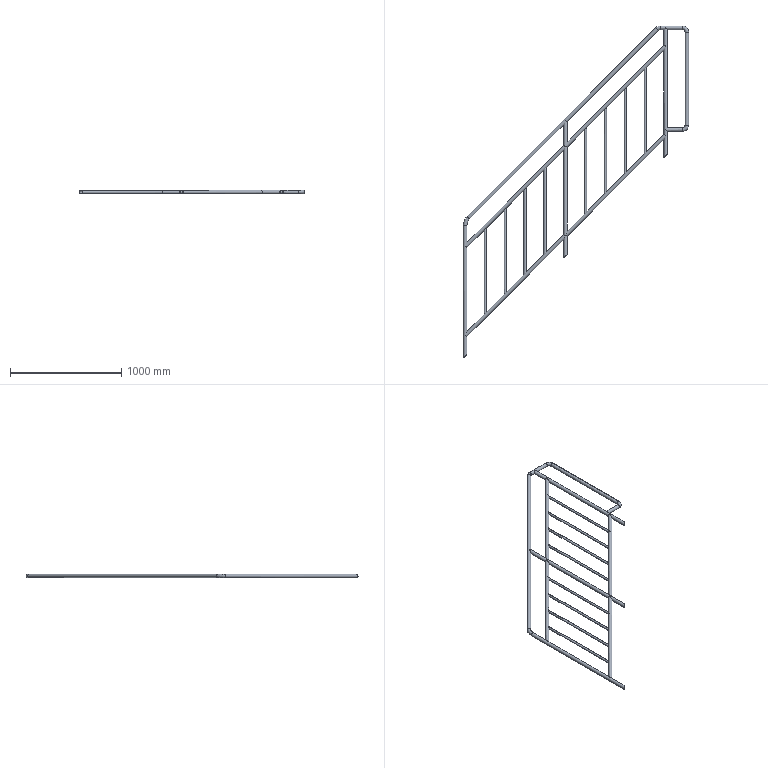Part | STEP file | PN_0012 stair guardrail B_Default<As Machined> | 23 solids | 92 faces | box 2022 x 2980 x 32 mm | volume 3009194 mm3 | cylinder 61 | plane 23 | torus 8 | commonest cylinder face diameters 32 x34 28 x11 16 x8 20 x8